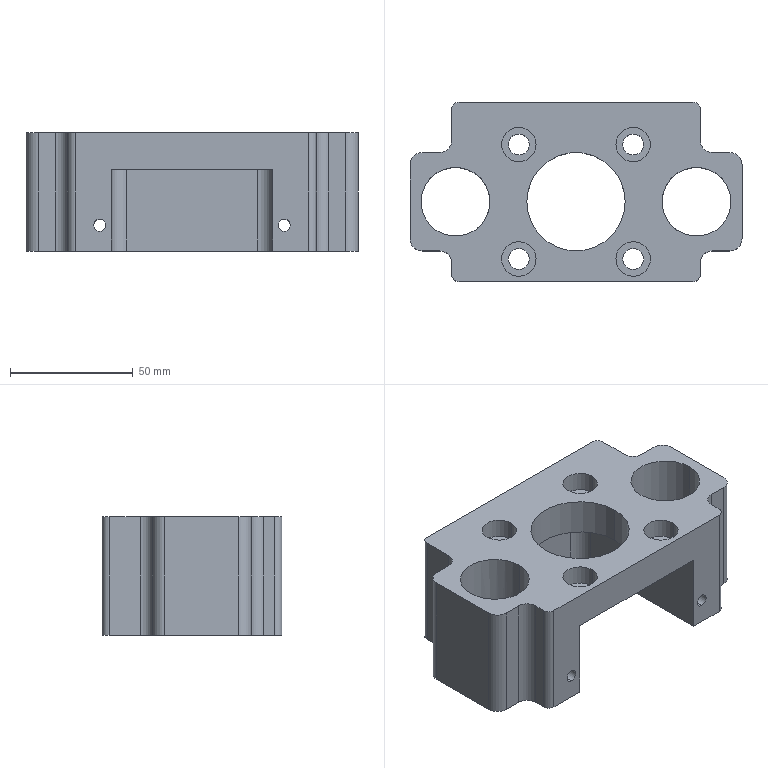Part | STEP file | 1 solid | 74 faces | box 135 x 73 x 48 mm | volume 191196 mm3 | cylinder 48 | plane 22 | cone 4 | commonest cylinder face diameters 5 x12 8.5 x8 10 x8 14 x8 6 x4 28 x4